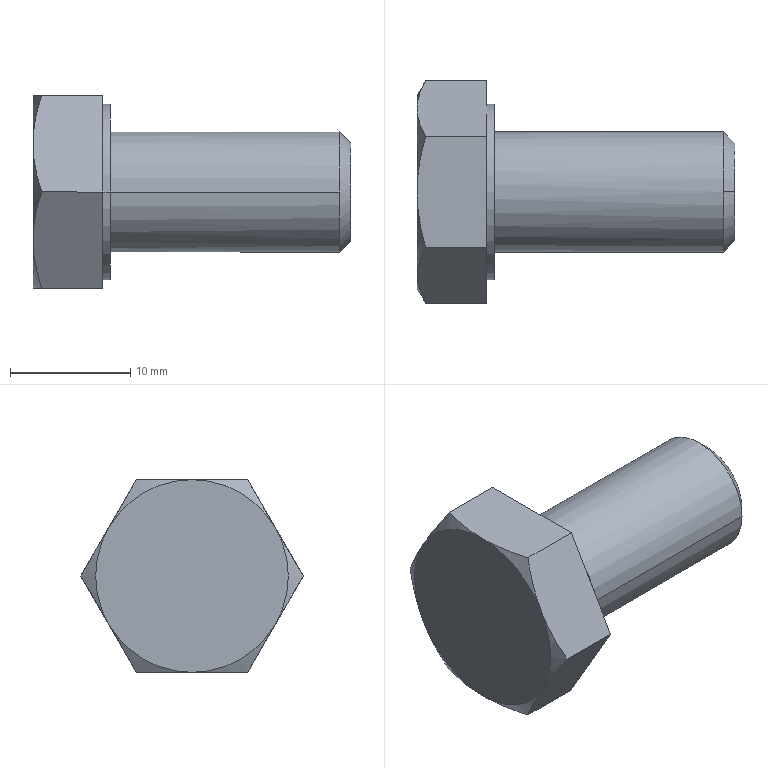Part | SolidWorks | features BaseBody 1 | 1 solid | 22 faces | box 26.4 x 18.475 x 16 mm | volume 2940 mm3 | plane 10 | cone 8 | cylinder 4 | commonest cylinder face diameters 10 x2 14.6 x2
STEP:
#1=CARTESIAN_POINT('',(0.,5.,0.));
#2=VERTEX_POINT('',#1);
#3=CARTESIAN_POINT('',(0.,-5.,0.));
#4=VERTEX_POINT('',#3);
#5=CARTESIAN_POINT('',(0.,0.,0.));
#6=DIRECTION('',(1.,0.,0.));
#7=DIRECTION('',(0.,1.,0.));
#8=AXIS2_PLACEMENT_3D('',#5,#6,#7);
#9=CIRCLE('',#8,5.);
#10=EDGE_CURVE('',#2,#4,#9,.T.);
#11=ORIENTED_EDGE('',*,*,#10,.T.);
#12=CARTESIAN_POINT('',(19.08,-5.,0.));
#13=VERTEX_POINT('',#12);
#14=CARTESIAN_POINT('',(10.75,-5.,0.));
#15=DIRECTION('',(1.,0.,0.));
#16=VECTOR('',#15,1000.);
#17=LINE('',#14,#16);
#18=EDGE_CURVE('',#4,#13,#17,.T.);
#19=ORIENTED_EDGE('',*,*,#18,.T.);
#20=CARTESIAN_POINT('',(19.08,0.,5.));
#21=VERTEX_POINT('',#20);
#22=CARTESIAN_POINT('',(19.08,0.,0.));
#23=DIRECTION('',(-1.,0.,0.));
#24=DIRECTION('',(0.,1.,0.));
#25=AXIS2_PLACEMENT_3D('',#22,#23,#24);
#26=CIRCLE('',#25,5.);
#27=EDGE_CURVE('',#13,#21,#26,.T.);
#28=ORIENTED_EDGE('',*,*,#27,.T.);
#29=CARTESIAN_POINT('',(19.08,5.,0.));
#30=VERTEX_POINT('',#29);
#31=CARTESIAN_POINT('',(19.08,0.,0.));
#32=DIRECTION('',(-1.,0.,0.));
#33=DIRECTION('',(0.,1.,0.));
#34=AXIS2_PLACEMENT_3D('',#31,#32,#33);
#35=CIRCLE('',#34,5.);
#36=EDGE_CURVE('',#21,#30,#35,.T.);
#37=ORIENTED_EDGE('',*,*,#36,.T.);
#38=CARTESIAN_POINT('',(10.75,5.,0.));
#39=DIRECTION('',(1.,0.,0.));
#40=VECTOR('',#39,1000.);
#41=LINE('',#38,#40);
#42=EDGE_CURVE('',#2,#30,#41,.T.);
#43=ORIENTED_EDGE('',*,*,#42,.F.);
#44=EDGE_LOOP('',(#11,#19,#28,#37,#43));
#45=FACE_OUTER_BOUND('',#44,.T.);
#46=CARTESIAN_POINT('',(10.75,0.,0.));
#47=DIRECTION('',(1.,0.,0.));
#48=DIRECTION('',(0.,1.,0.));
#49=AXIS2_PLACEMENT_3D('',#46,#47,#48);
#50=CYLINDRICAL_SURFACE('',#49,5.);
#51=ADVANCED_FACE('',(#45),#50,.T.);
#52=CARTESIAN_POINT('',(20.,0.,4.08));
#53=VERTEX_POINT('',#52);
#54=CARTESIAN_POINT('',(20.,0.,-4.08));
#55=VERTEX_POINT('',#54);
#56=CARTESIAN_POINT('',(20.,0.,0.));
#57=DIRECTION('',(-1.,0.,0.));
#58=DIRECTION('',(0.,0.,1.));
#59=AXIS2_PLACEMENT_3D('',#56,#57,#58);
#60=CIRCLE('',#59,4.08);
#61=EDGE_CURVE('',#53,#55,#60,.T.);
#62=ORIENTED_EDGE('',*,*,#61,.T.);
#63=CARTESIAN_POINT('',(19.08,0.,-5.));
#64=VERTEX_POINT('',#63);
#65=CARTESIAN_POINT('',(19.08,0.,-5.));
#66=DIRECTION('',(-0.7071,0.,-0.7071));
#67=VECTOR('',#66,1000.);
#68=LINE('',#65,#67);
#69=EDGE_CURVE('',#55,#64,#68,.T.);
#70=ORIENTED_EDGE('',*,*,#69,.T.);
#71=CARTESIAN_POINT('',(19.08,0.,0.));
#72=DIRECTION('',(-1.,0.,0.));
#73=DIRECTION('',(0.,1.,0.));
#74=AXIS2_PLACEMENT_3D('',#71,#72,#73);
#75=CIRCLE('',#74,5.);
#76=EDGE_CURVE('',#30,#64,#75,.T.);
#77=ORIENTED_EDGE('',*,*,#76,.F.);
#78=ORIENTED_EDGE('',*,*,#36,.F.);
#79=CARTESIAN_POINT('',(19.08,0.,5.));
#80=DIRECTION('',(-0.7071,0.,0.7071));
#81=VECTOR('',#80,1000.);
#82=LINE('',#79,#81);
#83=EDGE_CURVE('',#53,#21,#82,.T.);
#84=ORIENTED_EDGE('',*,*,#83,.F.);
#85=EDGE_LOOP('',(#62,#70,#77,#78,#84));
#86=FACE_OUTER_BOUND('',#85,.T.);
#87=CARTESIAN_POINT('',(19.08,0.,0.));
#88=DIRECTION('',(-1.,0.,0.));
#89=DIRECTION('',(0.,0.,1.));
#90=AXIS2_PLACEMENT_3D('',#87,#88,#89);
#91=CONICAL_SURFACE('',#90,5.,0.7853);
#92=ADVANCED_FACE('',(#86),#91,.T.);
#93=CARTESIAN_POINT('',(-0.6001,7.3,0.));
#94=VERTEX_POINT('',#93);
#95=CARTESIAN_POINT('',(-0.6001,-7.3,0.));
#96=VERTEX_POINT('',#95);
#97=CARTESIAN_POINT('',(-0.6001,0.,0.));
#98=DIRECTION('',(1.,0.,0.));
#99=DIRECTION('',(0.,1.,0.));
#100=AXIS2_PLACEMENT_3D('',#97,#98,#99);
#101=CIRCLE('',#100,7.3);
#102=EDGE_CURVE('',#94,#96,#101,.T.);
#103=ORIENTED_EDGE('',*,*,#102,.T.);
#104=CARTESIAN_POINT('',(0.,-7.3,0.));
#105=VERTEX_POINT('',#104);
#106=CARTESIAN_POINT('',(-0.3,-7.3,0.));
#107=DIRECTION('',(1.,0.,0.));
#108=VECTOR('',#107,1000.);
#109=LINE('',#106,#108);
#110=EDGE_CURVE('',#96,#105,#109,.T.);
#111=ORIENTED_EDGE('',*,*,#110,.T.);
#112=CARTESIAN_POINT('',(0.,7.3,0.));
#113=VERTEX_POINT('',#112);
#114=CARTESIAN_POINT('',(0.,0.,0.));
#115=DIRECTION('',(1.,0.,0.));
#116=DIRECTION('',(0.,1.,0.));
#117=AXIS2_PLACEMENT_3D('',#114,#115,#116);
#118=CIRCLE('',#117,7.3);
#119=EDGE_CURVE('',#113,#105,#118,.T.);
#120=ORIENTED_EDGE('',*,*,#119,.F.);
#121=CARTESIAN_POINT('',(-0.3,7.3,0.));
#122=DIRECTION('',(1.,0.,0.));
#123=VECTOR('',#122,1000.);
#124=LINE('',#121,#123);
#125=EDGE_CURVE('',#94,#113,#124,.T.);
#126=ORIENTED_EDGE('',*,*,#125,.F.);
#127=EDGE_LOOP('',(#103,#111,#120,#126));
#128=FACE_OUTER_BOUND('',#127,.T.);
#129=CARTESIAN_POINT('',(-0.3,0.,0.));
#130=DIRECTION('',(1.,0.,0.));
#131=DIRECTION('',(0.,1.,0.));
#132=AXIS2_PLACEMENT_3D('',#129,#130,#131);
#133=CYLINDRICAL_SURFACE('',#132,7.3);
#134=ADVANCED_FACE('',(#128),#133,.T.);
#135=ORIENTED_EDGE('',*,*,#18,.F.);
#136=CARTESIAN_POINT('',(0.,0.,0.));
#137=DIRECTION('',(1.,0.,0.));
#138=DIRECTION('',(0.,1.,0.));
#139=AXIS2_PLACEMENT_3D('',#136,#137,#138);
#140=CIRCLE('',#139,5.);
#141=EDGE_CURVE('',#4,#2,#140,.T.);
#142=ORIENTED_EDGE('',*,*,#141,.T.);
#143=ORIENTED_EDGE('',*,*,#42,.T.);
#144=ORIENTED_EDGE('',*,*,#76,.T.);
#145=CARTESIAN_POINT('',(19.08,0.,0.));
#146=DIRECTION('',(-1.,0.,0.));
#147=DIRECTION('',(0.,1.,0.));
#148=AXIS2_PLACEMENT_3D('',#145,#146,#147);
#149=CIRCLE('',#148,5.);
#150=EDGE_CURVE('',#64,#13,#149,.T.);
#151=ORIENTED_EDGE('',*,*,#150,.T.);
#152=EDGE_LOOP('',(#135,#142,#143,#144,#151));
#153=FACE_OUTER_BOUND('',#152,.T.);
#154=CARTESIAN_POINT('',(10.75,0.,0.));
#155=DIRECTION('',(1.,0.,0.));
#156=DIRECTION('',(0.,1.,0.));
#157=AXIS2_PLACEMENT_3D('',#154,#155,#156);
#158=CYLINDRICAL_SURFACE('',#157,5.);
#159=ADVANCED_FACE('',(#153),#158,.T.);
#160=ORIENTED_EDGE('',*,*,#69,.F.);
#161=CARTESIAN_POINT('',(20.,0.,0.));
#162=DIRECTION('',(-1.,0.,0.));
#163=DIRECTION('',(0.,0.,1.));
#164=AXIS2_PLACEMENT_3D('',#161,#162,#163);
#165=CIRCLE('',#164,4.08);
#166=EDGE_CURVE('',#55,#53,#165,.T.);
#167=ORIENTED_EDGE('',*,*,#166,.T.);
#168=ORIENTED_EDGE('',*,*,#83,.T.);
#169=ORIENTED_EDGE('',*,*,#27,.F.);
#170=ORIENTED_EDGE('',*,*,#150,.F.);
#171=EDGE_LOOP('',(#160,#167,#168,#169,#170));
#172=FACE_OUTER_BOUND('',#171,.T.);
#173=CARTESIAN_POINT('',(19.08,0.,0.));
#174=DIRECTION('',(-1.,0.,0.));
#175=DIRECTION('',(0.,0.,1.));
#176=AXIS2_PLACEMENT_3D('',#173,#174,#175);
#177=CONICAL_SURFACE('',#176,5.,0.7853);
#178=ADVANCED_FACE('',(#172),#177,.T.);
#179=ORIENTED_EDGE('',*,*,#10,.F.);
#180=ORIENTED_EDGE('',*,*,#141,.F.);
#181=EDGE_LOOP('',(#179,#180));
#182=FACE_BOUND('',#181,.T.);
#183=ORIENTED_EDGE('',*,*,#119,.T.);
#184=CARTESIAN_POINT('',(0.,0.,0.));
#185=DIRECTION('',(1.,0.,0.));
#186=DIRECTION('',(0.,1.,0.));
#187=AXIS2_PLACEMENT_3D('',#184,#185,#186);
#188=CIRCLE('',#187,7.3);
#189=EDGE_CURVE('',#105,#113,#188,.T.);
#190=ORIENTED_EDGE('',*,*,#189,.T.);
#191=EDGE_LOOP('',(#183,#190));
#192=FACE_OUTER_BOUND('',#191,.T.);
#193=CARTESIAN_POINT('',(0.,6.15,0.));
#194=DIRECTION('',(1.,0.,0.));
#195=DIRECTION('',(0.,1.,0.));
#196=AXIS2_PLACEMENT_3D('',#193,#194,#195);
#197=PLANE('',#196);
#198=ADVANCED_FACE('',(#182,#192),#197,.T.);
#199=ORIENTED_EDGE('',*,*,#61,.F.);
#200=ORIENTED_EDGE('',*,*,#166,.F.);
#201=EDGE_LOOP('',(#199,#200));
#202=FACE_OUTER_BOUND('',#201,.T.);
#203=CARTESIAN_POINT('',(20.,2.5,0.));
#204=DIRECTION('',(1.,0.,0.));
#205=DIRECTION('',(0.,1.,0.));
#206=AXIS2_PLACEMENT_3D('',#203,#204,#205);
#207=PLANE('',#206);
#208=ADVANCED_FACE('',(#202),#207,.T.);
#209=ORIENTED_EDGE('',*,*,#110,.F.);
#210=CARTESIAN_POINT('',(-0.6001,0.,0.));
#211=DIRECTION('',(1.,0.,0.));
#212=DIRECTION('',(0.,1.,0.));
#213=AXIS2_PLACEMENT_3D('',#210,#211,#212);
#214=CIRCLE('',#213,7.3);
#215=EDGE_CURVE('',#96,#94,#214,.T.);
#216=ORIENTED_EDGE('',*,*,#215,.T.);
#217=ORIENTED_EDGE('',*,*,#125,.T.);
#218=ORIENTED_EDGE('',*,*,#189,.F.);
#219=EDGE_LOOP('',(#209,#216,#217,#218));
#220=FACE_OUTER_BOUND('',#219,.T.);
#221=CARTESIAN_POINT('',(-0.3,0.,0.));
#222=DIRECTION('',(1.,0.,0.));
#223=DIRECTION('',(0.,1.,0.));
#224=AXIS2_PLACEMENT_3D('',#221,#222,#223);
#225=CYLINDRICAL_SURFACE('',#224,7.3);
#226=ADVANCED_FACE('',(#220),#225,.T.);
#227=ORIENTED_EDGE('',*,*,#102,.F.);
#228=ORIENTED_EDGE('',*,*,#215,.F.);
#229=EDGE_LOOP('',(#227,#228));
#230=FACE_BOUND('',#229,.T.);
#231=CARTESIAN_POINT('',(-0.6001,-4.619,-8.));
#232=VERTEX_POINT('',#231);
#233=CARTESIAN_POINT('',(-0.6001,4.619,-8.));
#234=VERTEX_POINT('',#233);
#235=CARTESIAN_POINT('',(-0.6001,0.,-8.));
#236=DIRECTION('',(0.,1.,0.));
#237=VECTOR('',#236,1000.);
#238=LINE('',#235,#237);
#239=EDGE_CURVE('',#232,#234,#238,.T.);
#240=ORIENTED_EDGE('',*,*,#239,.T.);
#241=CARTESIAN_POINT('',(-0.6001,9.238,0.));
#242=VERTEX_POINT('',#241);
#243=CARTESIAN_POINT('',(-0.6001,4.619,-8.));
#244=DIRECTION('',(0.,0.5,0.866));
#245=VECTOR('',#244,1000.);
#246=LINE('',#243,#245);
#247=EDGE_CURVE('',#234,#242,#246,.T.);
#248=ORIENTED_EDGE('',*,*,#247,.T.);
#249=CARTESIAN_POINT('',(-0.6001,4.619,8.));
#250=VERTEX_POINT('',#249);
#251=CARTESIAN_POINT('',(-0.6001,9.238,0.));
#252=DIRECTION('',(0.,-0.5,0.866));
#253=VECTOR('',#252,1000.);
#254=LINE('',#251,#253);
#255=EDGE_CURVE('',#242,#250,#254,.T.);
#256=ORIENTED_EDGE('',*,*,#255,.T.);
#257=CARTESIAN_POINT('',(-0.6001,-4.619,8.));
#258=VERTEX_POINT('',#257);
#259=CARTESIAN_POINT('',(-0.6001,0.,8.));
#260=DIRECTION('',(0.,-1.,0.));
#261=VECTOR('',#260,1000.);
#262=LINE('',#259,#261);
#263=EDGE_CURVE('',#250,#258,#262,.T.);
#264=ORIENTED_EDGE('',*,*,#263,.T.);
#265=CARTESIAN_POINT('',(-0.6001,-9.238,0.));
#266=VERTEX_POINT('',#265);
#267=CARTESIAN_POINT('',(-0.6001,-4.619,8.));
#268=DIRECTION('',(0.,-0.5,-0.866));
#269=VECTOR('',#268,1000.);
#270=LINE('',#267,#269);
#271=EDGE_CURVE('',#258,#266,#270,.T.);
#272=ORIENTED_EDGE('',*,*,#271,.T.);
#273=CARTESIAN_POINT('',(-0.6001,-9.238,0.));
#274=DIRECTION('',(0.,0.5,-0.866));
#275=VECTOR('',#274,1000.);
#276=LINE('',#273,#275);
#277=EDGE_CURVE('',#266,#232,#276,.T.);
#278=ORIENTED_EDGE('',*,*,#277,.T.);
#279=EDGE_LOOP('',(#240,#248,#256,#264,#272,#278));
#280=FACE_OUTER_BOUND('',#279,.T.);
#281=CARTESIAN_POINT('',(-0.6001,0.,0.));
#282=DIRECTION('',(1.,0.,0.));
#283=DIRECTION('',(0.,1.,0.));
#284=AXIS2_PLACEMENT_3D('',#281,#282,#283);
#285=PLANE('',#284);
#286=ADVANCED_FACE('',(#230,#280),#285,.T.);
#287=ORIENTED_EDGE('',*,*,#247,.F.);
#288=CARTESIAN_POINT('',(-5.686,4.619,-8.));
#289=VERTEX_POINT('',#288);
#290=CARTESIAN_POINT('',(-0.6001,4.619,-8.));
#291=DIRECTION('',(-1.,0.,0.));
#292=VECTOR('',#291,1000.);
#293=LINE('',#290,#292);
#294=EDGE_CURVE('',#234,#289,#293,.T.);
#295=ORIENTED_EDGE('',*,*,#294,.T.);
#296=CARTESIAN_POINT('',(-6.4,6.928,-4.));
#297=VERTEX_POINT('',#296);
#298=CARTESIAN_POINT('',(-5.686,4.619,-8.));
#299=CARTESIAN_POINT('',(-5.903,4.996,-7.347));
#300=CARTESIAN_POINT('',(-6.083,5.376,-6.688));
#301=CARTESIAN_POINT('',(-6.332,6.145,-5.356));
#302=CARTESIAN_POINT('',(-6.4,6.534,-4.683));
#303=CARTESIAN_POINT('',(-6.4,6.928,-4.));
#304=B_SPLINE_CURVE_WITH_KNOTS('',3,(#298,#299,#300,#301,#302,#303),.UNSPECIFIED.,.F.,.F.,(4,2,4),(0.,0.002337,0.004674),.UNSPECIFIED.);
#305=EDGE_CURVE('',#289,#297,#304,.T.);
#306=ORIENTED_EDGE('',*,*,#305,.T.);
#307=CARTESIAN_POINT('',(-5.686,9.238,0.));
#308=VERTEX_POINT('',#307);
#309=CARTESIAN_POINT('',(-6.4,6.928,-4.));
#310=CARTESIAN_POINT('',(-6.4,7.322,-3.317));
#311=CARTESIAN_POINT('',(-6.332,7.711,-2.644));
#312=CARTESIAN_POINT('',(-6.083,8.48,-1.312));
#313=CARTESIAN_POINT('',(-5.903,8.86,-0.6534));
#314=CARTESIAN_POINT('',(-5.686,9.238,0.));
#315=B_SPLINE_CURVE_WITH_KNOTS('',3,(#309,#310,#311,#312,#313,#314),.UNSPECIFIED.,.F.,.F.,(4,2,4),(0.,0.002337,0.004674),.UNSPECIFIED.);
#316=EDGE_CURVE('',#297,#308,#315,.T.);
#317=ORIENTED_EDGE('',*,*,#316,.T.);
#318=CARTESIAN_POINT('',(-0.6001,9.238,0.));
#319=DIRECTION('',(1.,0.,0.));
#320=VECTOR('',#319,1000.);
#321=LINE('',#318,#320);
#322=EDGE_CURVE('',#308,#242,#321,.T.);
#323=ORIENTED_EDGE('',*,*,#322,.T.);
#324=EDGE_LOOP('',(#287,#295,#306,#317,#323));
#325=FACE_OUTER_BOUND('',#324,.T.);
#326=CARTESIAN_POINT('',(-0.6001,4.619,-8.));
#327=DIRECTION('',(0.,0.866,-0.5));
#328=DIRECTION('',(0.,0.5,0.866));
#329=AXIS2_PLACEMENT_3D('',#326,#327,#328);
#330=PLANE('',#329);
#331=ADVANCED_FACE('',(#325),#330,.T.);
#332=ORIENTED_EDGE('',*,*,#239,.F.);
#333=CARTESIAN_POINT('',(-5.686,-4.619,-8.));
#334=VERTEX_POINT('',#333);
#335=CARTESIAN_POINT('',(-0.6001,-4.619,-8.));
#336=DIRECTION('',(-1.,0.,0.));
#337=VECTOR('',#336,1000.);
#338=LINE('',#335,#337);
#339=EDGE_CURVE('',#232,#334,#338,.T.);
#340=ORIENTED_EDGE('',*,*,#339,.T.);
#341=CARTESIAN_POINT('',(-6.4,0.,-8.));
#342=VERTEX_POINT('',#341);
#343=CARTESIAN_POINT('',(-5.686,-4.619,-8.));
#344=CARTESIAN_POINT('',(-5.903,-3.864,-8.));
#345=CARTESIAN_POINT('',(-6.083,-3.104,-8.));
#346=CARTESIAN_POINT('',(-6.332,-1.566,-8.));
#347=CARTESIAN_POINT('',(-6.4,-0.7882,-8.));
#348=CARTESIAN_POINT('',(-6.4,0.,-8.));
#349=B_SPLINE_CURVE_WITH_KNOTS('',3,(#343,#344,#345,#346,#347,#348),.UNSPECIFIED.,.F.,.F.,(4,2,4),(0.,0.002337,0.004674),.UNSPECIFIED.);
#350=EDGE_CURVE('',#334,#342,#349,.T.);
#351=ORIENTED_EDGE('',*,*,#350,.T.);
#352=CARTESIAN_POINT('',(-6.4,0.,-8.));
#353=CARTESIAN_POINT('',(-6.4,0.7882,-8.));
#354=CARTESIAN_POINT('',(-6.332,1.566,-8.));
#355=CARTESIAN_POINT('',(-6.083,3.104,-8.));
#356=CARTESIAN_POINT('',(-5.903,3.864,-8.));
#357=CARTESIAN_POINT('',(-5.686,4.619,-8.));
#358=B_SPLINE_CURVE_WITH_KNOTS('',3,(#352,#353,#354,#355,#356,#357),.UNSPECIFIED.,.F.,.F.,(4,2,4),(0.,0.002337,0.004674),.UNSPECIFIED.);
#359=EDGE_CURVE('',#342,#289,#358,.T.);
#360=ORIENTED_EDGE('',*,*,#359,.T.);
#361=ORIENTED_EDGE('',*,*,#294,.F.);
#362=EDGE_LOOP('',(#332,#340,#351,#360,#361));
#363=FACE_OUTER_BOUND('',#362,.T.);
#364=CARTESIAN_POINT('',(-0.6001,-4.619,-8.));
#365=DIRECTION('',(0.,0.,-1.));
#366=DIRECTION('',(0.,1.,0.));
#367=AXIS2_PLACEMENT_3D('',#364,#365,#366);
#368=PLANE('',#367);
#369=ADVANCED_FACE('',(#363),#368,.T.);
#370=CARTESIAN_POINT('',(-5.686,-9.238,0.));
#371=VERTEX_POINT('',#370);
#372=CARTESIAN_POINT('',(-0.6001,-9.238,0.));
#373=DIRECTION('',(-1.,0.,0.));
#374=VECTOR('',#373,1000.);
#375=LINE('',#372,#374);
#376=EDGE_CURVE('',#266,#371,#375,.T.);
#377=ORIENTED_EDGE('',*,*,#376,.T.);
#378=CARTESIAN_POINT('',(-6.4,-6.928,-4.));
#379=VERTEX_POINT('',#378);
#380=CARTESIAN_POINT('',(-5.686,-9.238,0.));
#381=CARTESIAN_POINT('',(-5.903,-8.86,-0.6534));
#382=CARTESIAN_POINT('',(-6.083,-8.48,-1.312));
#383=CARTESIAN_POINT('',(-6.332,-7.711,-2.644));
#384=CARTESIAN_POINT('',(-6.4,-7.322,-3.317));
#385=CARTESIAN_POINT('',(-6.4,-6.928,-4.));
#386=B_SPLINE_CURVE_WITH_KNOTS('',3,(#380,#381,#382,#383,#384,#385),.UNSPECIFIED.,.F.,.F.,(4,2,4),(0.,0.002337,0.004674),.UNSPECIFIED.);
#387=EDGE_CURVE('',#371,#379,#386,.T.);
#388=ORIENTED_EDGE('',*,*,#387,.T.);
#389=CARTESIAN_POINT('',(-6.4,-6.928,-4.));
#390=CARTESIAN_POINT('',(-6.4,-6.534,-4.683));
#391=CARTESIAN_POINT('',(-6.332,-6.145,-5.356));
#392=CARTESIAN_POINT('',(-6.083,-5.376,-6.688));
#393=CARTESIAN_POINT('',(-5.903,-4.996,-7.347));
#394=CARTESIAN_POINT('',(-5.686,-4.619,-8.));
#395=B_SPLINE_CURVE_WITH_KNOTS('',3,(#389,#390,#391,#392,#393,#394),.UNSPECIFIED.,.F.,.F.,(4,2,4),(0.,0.002337,0.004674),.UNSPECIFIED.);
#396=EDGE_CURVE('',#379,#334,#395,.T.);
#397=ORIENTED_EDGE('',*,*,#396,.T.);
#398=ORIENTED_EDGE('',*,*,#339,.F.);
#399=ORIENTED_EDGE('',*,*,#277,.F.);
#400=EDGE_LOOP('',(#377,#388,#397,#398,#399));
#401=FACE_OUTER_BOUND('',#400,.T.);
#402=CARTESIAN_POINT('',(-0.6001,-9.238,0.));
#403=DIRECTION('',(0.,-0.866,-0.5));
#404=DIRECTION('',(0.,0.5,-0.866));
#405=AXIS2_PLACEMENT_3D('',#402,#403,#404);
#406=PLANE('',#405);
#407=ADVANCED_FACE('',(#401),#406,.T.);
#408=CARTESIAN_POINT('',(-5.686,-4.619,8.));
#409=VERTEX_POINT('',#408);
#410=CARTESIAN_POINT('',(-0.6001,-4.619,8.));
#411=DIRECTION('',(-1.,0.,0.));
#412=VECTOR('',#411,1000.);
#413=LINE('',#410,#412);
#414=EDGE_CURVE('',#258,#409,#413,.T.);
#415=ORIENTED_EDGE('',*,*,#414,.T.);
#416=CARTESIAN_POINT('',(-6.4,-6.928,4.));
#417=VERTEX_POINT('',#416);
#418=CARTESIAN_POINT('',(-5.686,-4.619,8.));
#419=CARTESIAN_POINT('',(-5.903,-4.996,7.347));
#420=CARTESIAN_POINT('',(-6.083,-5.376,6.688));
#421=CARTESIAN_POINT('',(-6.332,-6.145,5.356));
#422=CARTESIAN_POINT('',(-6.4,-6.534,4.683));
#423=CARTESIAN_POINT('',(-6.4,-6.928,4.));
#424=B_SPLINE_CURVE_WITH_KNOTS('',3,(#418,#419,#420,#421,#422,#423),.UNSPECIFIED.,.F.,.F.,(4,2,4),(0.,0.002337,0.004674),.UNSPECIFIED.);
#425=EDGE_CURVE('',#409,#417,#424,.T.);
#426=ORIENTED_EDGE('',*,*,#425,.T.);
#427=CARTESIAN_POINT('',(-6.4,-6.928,4.));
#428=CARTESIAN_POINT('',(-6.4,-7.322,3.317));
#429=CARTESIAN_POINT('',(-6.332,-7.711,2.644));
#430=CARTESIAN_POINT('',(-6.083,-8.48,1.312));
#431=CARTESIAN_POINT('',(-5.903,-8.86,0.6534));
#432=CARTESIAN_POINT('',(-5.686,-9.238,0.));
#433=B_SPLINE_CURVE_WITH_KNOTS('',3,(#427,#428,#429,#430,#431,#432),.UNSPECIFIED.,.F.,.F.,(4,2,4),(0.,0.002337,0.004674),.UNSPECIFIED.);
#434=EDGE_CURVE('',#417,#371,#433,.T.);
#435=ORIENTED_EDGE('',*,*,#434,.T.);
#436=ORIENTED_EDGE('',*,*,#376,.F.);
#437=ORIENTED_EDGE('',*,*,#271,.F.);
#438=EDGE_LOOP('',(#415,#426,#435,#436,#437));
#439=FACE_OUTER_BOUND('',#438,.T.);
#440=CARTESIAN_POINT('',(-0.6001,-4.619,8.));
#441=DIRECTION('',(0.,-0.866,0.5));
#442=DIRECTION('',(0.,-0.5,-0.866));
#443=AXIS2_PLACEMENT_3D('',#440,#441,#442);
#444=PLANE('',#443);
#445=ADVANCED_FACE('',(#439),#444,.T.);
#446=CARTESIAN_POINT('',(-5.686,4.619,8.));
#447=VERTEX_POINT('',#446);
#448=CARTESIAN_POINT('',(-0.6001,4.619,8.));
#449=DIRECTION('',(-1.,0.,0.));
#450=VECTOR('',#449,1000.);
#451=LINE('',#448,#450);
#452=EDGE_CURVE('',#250,#447,#451,.T.);
#453=ORIENTED_EDGE('',*,*,#452,.T.);
#454=CARTESIAN_POINT('',(-6.4,0.,8.));
#455=VERTEX_POINT('',#454);
#456=CARTESIAN_POINT('',(-5.686,4.619,8.));
#457=CARTESIAN_POINT('',(-5.903,3.864,8.));
#458=CARTESIAN_POINT('',(-6.083,3.104,8.));
#459=CARTESIAN_POINT('',(-6.332,1.566,8.));
#460=CARTESIAN_POINT('',(-6.4,0.7882,8.));
#461=CARTESIAN_POINT('',(-6.4,0.,8.));
#462=B_SPLINE_CURVE_WITH_KNOTS('',3,(#456,#457,#458,#459,#460,#461),.UNSPECIFIED.,.F.,.F.,(4,2,4),(0.,0.002337,0.004674),.UNSPECIFIED.);
#463=EDGE_CURVE('',#447,#455,#462,.T.);
#464=ORIENTED_EDGE('',*,*,#463,.T.);
#465=CARTESIAN_POINT('',(-6.4,0.,8.));
#466=CARTESIAN_POINT('',(-6.4,-0.7882,8.));
#467=CARTESIAN_POINT('',(-6.332,-1.566,8.));
#468=CARTESIAN_POINT('',(-6.083,-3.104,8.));
#469=CARTESIAN_POINT('',(-5.903,-3.864,8.));
#470=CARTESIAN_POINT('',(-5.686,-4.619,8.));
#471=B_SPLINE_CURVE_WITH_KNOTS('',3,(#465,#466,#467,#468,#469,#470),.UNSPECIFIED.,.F.,.F.,(4,2,4),(0.,0.002337,0.004674),.UNSPECIFIED.);
#472=EDGE_CURVE('',#455,#409,#471,.T.);
#473=ORIENTED_EDGE('',*,*,#472,.T.);
#474=ORIENTED_EDGE('',*,*,#414,.F.);
#475=ORIENTED_EDGE('',*,*,#263,.F.);
#476=EDGE_LOOP('',(#453,#464,#473,#474,#475));
#477=FACE_OUTER_BOUND('',#476,.T.);
#478=CARTESIAN_POINT('',(-0.6001,4.619,8.));
#479=DIRECTION('',(0.,0.,1.));
#480=DIRECTION('',(0.,-1.,0.));
#481=AXIS2_PLACEMENT_3D('',#478,#479,#480);
#482=PLANE('',#481);
#483=ADVANCED_FACE('',(#477),#482,.T.);
#484=ORIENTED_EDGE('',*,*,#255,.F.);
#485=ORIENTED_EDGE('',*,*,#322,.F.);
#486=CARTESIAN_POINT('',(-6.4,6.928,4.));
#487=VERTEX_POINT('',#486);
#488=CARTESIAN_POINT('',(-5.686,9.238,0.));
#489=CARTESIAN_POINT('',(-5.903,8.86,0.6534));
#490=CARTESIAN_POINT('',(-6.083,8.48,1.312));
#491=CARTESIAN_POINT('',(-6.332,7.711,2.644));
#492=CARTESIAN_POINT('',(-6.4,7.322,3.317));
#493=CARTESIAN_POINT('',(-6.4,6.928,4.));
#494=B_SPLINE_CURVE_WITH_KNOTS('',3,(#488,#489,#490,#491,#492,#493),.UNSPECIFIED.,.F.,.F.,(4,2,4),(0.,0.002337,0.004674),.UNSPECIFIED.);
#495=EDGE_CURVE('',#308,#487,#494,.T.);
#496=ORIENTED_EDGE('',*,*,#495,.T.);
#497=CARTESIAN_POINT('',(-6.4,6.928,4.));
#498=CARTESIAN_POINT('',(-6.4,6.534,4.683));
#499=CARTESIAN_POINT('',(-6.332,6.145,5.356));
#500=CARTESIAN_POINT('',(-6.083,5.376,6.688));
#501=CARTESIAN_POINT('',(-5.903,4.996,7.347));
#502=CARTESIAN_POINT('',(-5.686,4.619,8.));
#503=B_SPLINE_CURVE_WITH_KNOTS('',3,(#497,#498,#499,#500,#501,#502),.UNSPECIFIED.,.F.,.F.,(4,2,4),(0.,0.002337,0.004674),.UNSPECIFIED.);
#504=EDGE_CURVE('',#487,#447,#503,.T.);
#505=ORIENTED_EDGE('',*,*,#504,.T.);
#506=ORIENTED_EDGE('',*,*,#452,.F.);
#507=EDGE_LOOP('',(#484,#485,#496,#505,#506));
#508=FACE_OUTER_BOUND('',#507,.T.);
#509=CARTESIAN_POINT('',(-0.6001,9.238,0.));
#510=DIRECTION('',(0.,0.866,0.5));
#511=DIRECTION('',(0.,-0.5,0.866));
#512=AXIS2_PLACEMENT_3D('',#509,#510,#511);
#513=PLANE('',#512);
#514=ADVANCED_FACE('',(#508),#513,.T.);
#515=CARTESIAN_POINT('',(-6.4,0.,0.));
#516=DIRECTION('',(1.,0.,0.));
#517=DIRECTION('',(0.,0.,-1.));
#518=AXIS2_PLACEMENT_3D('',#515,#516,#517);
#519=CIRCLE('',#518,8.);
#520=EDGE_CURVE('',#297,#487,#519,.T.);
#521=ORIENTED_EDGE('',*,*,#520,.T.);
#522=ORIENTED_EDGE('',*,*,#495,.F.);
#523=ORIENTED_EDGE('',*,*,#316,.F.);
#524=EDGE_LOOP('',(#521,#522,#523));
#525=FACE_OUTER_BOUND('',#524,.T.);
#526=CARTESIAN_POINT('',(-5.681,0.,0.));
#527=DIRECTION('',(1.,0.,0.));
#528=DIRECTION('',(0.,0.,-1.));
#529=AXIS2_PLACEMENT_3D('',#526,#527,#528);
#530=CONICAL_SURFACE('',#529,9.245,1.047);
#531=ADVANCED_FACE('',(#525),#530,.T.);
#532=CARTESIAN_POINT('',(-6.4,0.,0.));
#533=DIRECTION('',(1.,0.,0.));
#534=DIRECTION('',(0.,0.,-1.));
#535=AXIS2_PLACEMENT_3D('',#532,#533,#534);
#536=CIRCLE('',#535,8.);
#537=EDGE_CURVE('',#342,#297,#536,.T.);
#538=ORIENTED_EDGE('',*,*,#537,.T.);
#539=ORIENTED_EDGE('',*,*,#305,.F.);
#540=ORIENTED_EDGE('',*,*,#359,.F.);
#541=EDGE_LOOP('',(#538,#539,#540));
#542=FACE_OUTER_BOUND('',#541,.T.);
#543=CARTESIAN_POINT('',(-5.681,0.,0.));
#544=DIRECTION('',(1.,0.,0.));
#545=DIRECTION('',(0.,0.,-1.));
#546=AXIS2_PLACEMENT_3D('',#543,#544,#545);
#547=CONICAL_SURFACE('',#546,9.245,1.047);
#548=ADVANCED_FACE('',(#542),#547,.T.);
#549=ORIENTED_EDGE('',*,*,#396,.F.);
#550=CARTESIAN_POINT('',(-6.4,0.,0.));
#551=DIRECTION('',(1.,0.,0.));
#552=DIRECTION('',(0.,0.,-1.));
#553=AXIS2_PLACEMENT_3D('',#550,#551,#552);
#554=CIRCLE('',#553,8.);
#555=EDGE_CURVE('',#379,#342,#554,.T.);
#556=ORIENTED_EDGE('',*,*,#555,.T.);
#557=ORIENTED_EDGE('',*,*,#350,.F.);
#558=EDGE_LOOP('',(#549,#556,#557));
#559=FACE_OUTER_BOUND('',#558,.T.);
#560=CARTESIAN_POINT('',(-5.681,0.,0.));
#561=DIRECTION('',(1.,0.,0.));
#562=DIRECTION('',(0.,0.,-1.));
#563=AXIS2_PLACEMENT_3D('',#560,#561,#562);
#564=CONICAL_SURFACE('',#563,9.245,1.047);
#565=ADVANCED_FACE('',(#559),#564,.T.);
#566=ORIENTED_EDGE('',*,*,#434,.F.);
#567=CARTESIAN_POINT('',(-6.4,0.,0.));
#568=DIRECTION('',(1.,0.,0.));
#569=DIRECTION('',(0.,0.,-1.));
#570=AXIS2_PLACEMENT_3D('',#567,#568,#569);
#571=CIRCLE('',#570,8.);
#572=EDGE_CURVE('',#417,#379,#571,.T.);
#573=ORIENTED_EDGE('',*,*,#572,.T.);
#574=ORIENTED_EDGE('',*,*,#387,.F.);
#575=EDGE_LOOP('',(#566,#573,#574));
#576=FACE_OUTER_BOUND('',#575,.T.);
#577=CARTESIAN_POINT('',(-5.681,0.,0.));
#578=DIRECTION('',(1.,0.,0.));
#579=DIRECTION('',(0.,0.,-1.));
#580=AXIS2_PLACEMENT_3D('',#577,#578,#579);
#581=CONICAL_SURFACE('',#580,9.245,1.047);
#582=ADVANCED_FACE('',(#576),#581,.T.);
#583=ORIENTED_EDGE('',*,*,#472,.F.);
#584=CARTESIAN_POINT('',(-6.4,0.,0.));
#585=DIRECTION('',(1.,0.,0.));
#586=DIRECTION('',(0.,0.,-1.));
#587=AXIS2_PLACEMENT_3D('',#584,#585,#586);
#588=CIRCLE('',#587,8.);
#589=EDGE_CURVE('',#455,#417,#588,.T.);
#590=ORIENTED_EDGE('',*,*,#589,.T.);
#591=ORIENTED_EDGE('',*,*,#425,.F.);
#592=EDGE_LOOP('',(#583,#590,#591));
#593=FACE_OUTER_BOUND('',#592,.T.);
#594=CARTESIAN_POINT('',(-5.681,0.,0.));
#595=DIRECTION('',(1.,0.,0.));
#596=DIRECTION('',(0.,0.,-1.));
#597=AXIS2_PLACEMENT_3D('',#594,#595,#596);
#598=CONICAL_SURFACE('',#597,9.245,1.047);
#599=ADVANCED_FACE('',(#593),#598,.T.);
#600=CARTESIAN_POINT('',(-6.4,0.,0.));
#601=DIRECTION('',(1.,0.,0.));
#602=DIRECTION('',(0.,0.,-1.));
#603=AXIS2_PLACEMENT_3D('',#600,#601,#602);
#604=CIRCLE('',#603,8.);
#605=EDGE_CURVE('',#487,#455,#604,.T.);
#606=ORIENTED_EDGE('',*,*,#605,.T.);
#607=ORIENTED_EDGE('',*,*,#463,.F.);
#608=ORIENTED_EDGE('',*,*,#504,.F.);
#609=EDGE_LOOP('',(#606,#607,#608));
#610=FACE_OUTER_BOUND('',#609,.T.);
#611=CARTESIAN_POINT('',(-5.681,0.,0.));
#612=DIRECTION('',(1.,0.,0.));
#613=DIRECTION('',(0.,0.,-1.));
#614=AXIS2_PLACEMENT_3D('',#611,#612,#613);
#615=CONICAL_SURFACE('',#614,9.245,1.047);
#616=ADVANCED_FACE('',(#610),#615,.T.);
#617=ORIENTED_EDGE('',*,*,#520,.F.);
#618=ORIENTED_EDGE('',*,*,#537,.F.);
#619=ORIENTED_EDGE('',*,*,#555,.F.);
#620=ORIENTED_EDGE('',*,*,#572,.F.);
#621=ORIENTED_EDGE('',*,*,#589,.F.);
#622=ORIENTED_EDGE('',*,*,#605,.F.);
#623=EDGE_LOOP('',(#617,#618,#619,#620,#621,#622));
#624=FACE_OUTER_BOUND('',#623,.T.);
#625=CARTESIAN_POINT('',(-6.4,0.,0.));
#626=DIRECTION('',(1.,0.,0.));
#627=DIRECTION('',(0.,1.,0.));
#628=AXIS2_PLACEMENT_3D('',#625,#626,#627);
#629=PLANE('',#628);
#630=ADVANCED_FACE('',(#624),#629,.F.);
#631=CLOSED_SHELL('',(#51,#92,#134,#159,#178,#198,#208,#226,#286,#331,#369,#407,#445,#483,#514,#531,#548,#565,#582,#599,#616,#630));
#632=MANIFOLD_SOLID_BREP('',#631);
#633=CARTESIAN_POINT('',(0.,0.,0.));
#634=DIRECTION('',(0.,0.,1.));
#635=DIRECTION('',(1.,0.,0.));
#636=AXIS2_PLACEMENT_3D('',#633,#634,#635);
#637=(LENGTH_UNIT()NAMED_UNIT(*)SI_UNIT(.MILLI.,.METRE.));
#638=UNCERTAINTY_MEASURE_WITH_UNIT(LENGTH_MEASURE(0.00001),#637,'','');
#639=(NAMED_UNIT(*)PLANE_ANGLE_UNIT()SI_UNIT($,.RADIAN.));
#640=(NAMED_UNIT(*)SI_UNIT($,.STERADIAN.)SOLID_ANGLE_UNIT());
#641=(GEOMETRIC_REPRESENTATION_CONTEXT(3)GLOBAL_UNCERTAINTY_ASSIGNED_CONTEXT((#638))GLOBAL_UNIT_ASSIGNED_CONTEXT((#637,#639,#640))REPRESENTATION_CONTEXT('',''));
#642=ADVANCED_BREP_SHAPE_REPRESENTATION('',(#632,#636),#641);